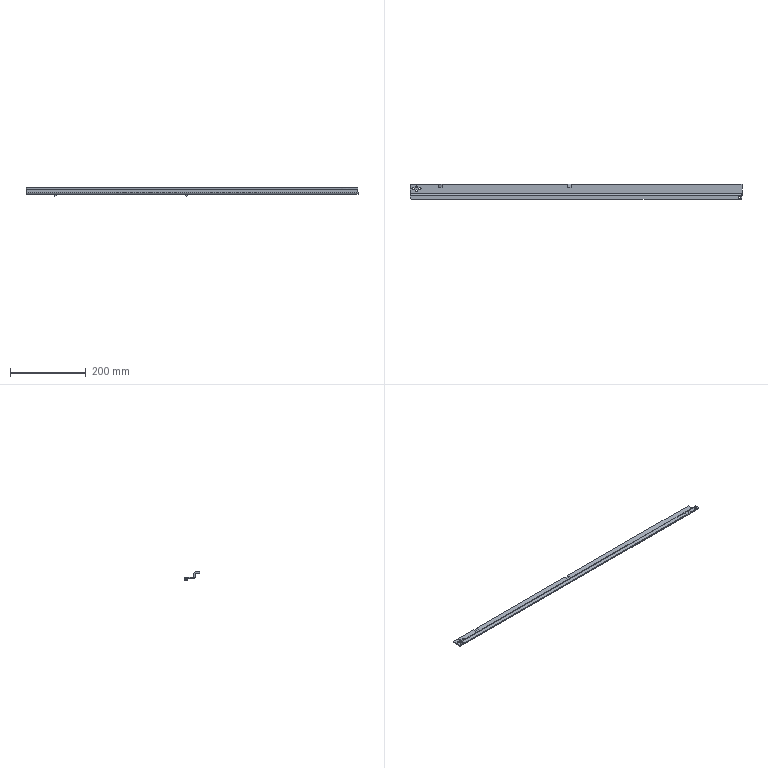Part | SolidWorks | features ICE 3, EdgeFlange 2, FormToolInstance 2, SMBaseFlange 2, Fillet 1, FlatPattern 1, SheetMetal 1 | 1 solid | 56 faces | box 875 x 40 x 21.683 mm | volume 132017 mm3 | plane 40 | cylinder 16 | commonest cylinder face diameters 6 x6 4 x4 3 x2 9 x2 10 x1 79.402 x1